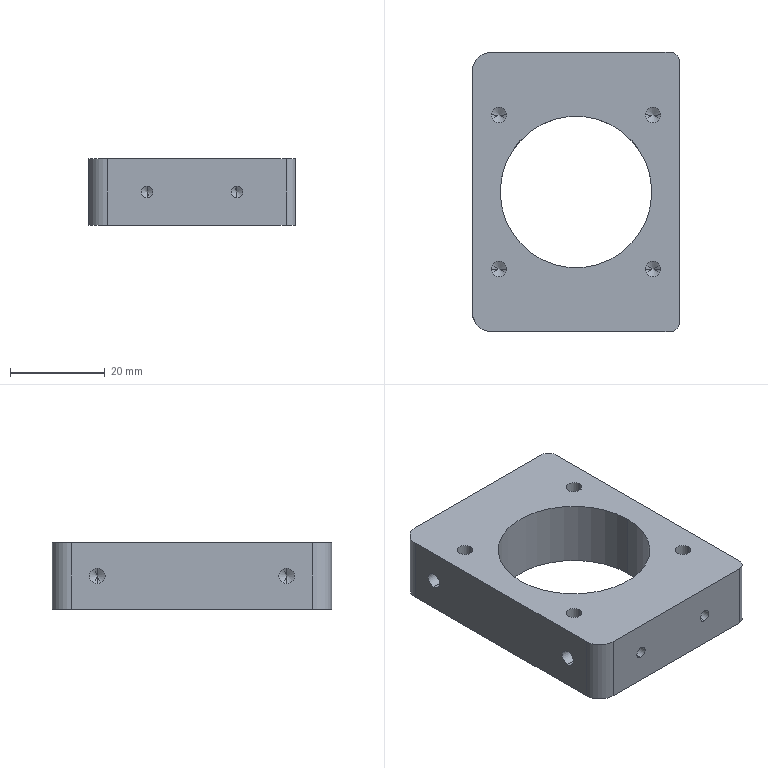Part | STEP file | 1 solid | 76 faces | box 43.7 x 59 x 14 mm | volume 23699 mm3 | cylinder 38 | cone 32 | plane 6 | commonest cylinder face diameters 2.5 x16 3.3 x16 4 x2 8 x2 32 x2